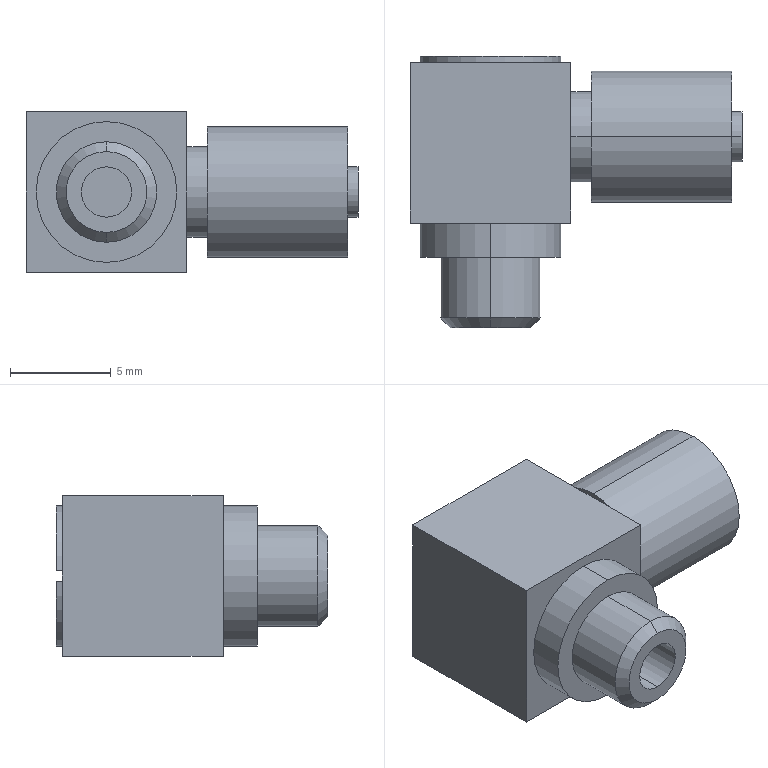Part | SolidWorks | features BaseBody 1, MoveCopyBody 1 | 1 solid | 39 faces | box 16.5 x 13.5 x 8 mm | volume 829.104 mm3 | plane 20 | cylinder 17 | cone 2 | commonest cylinder face diameters 7 x5 2.5 x4 1.8 x2 4.5 x2 5 x2 6.5 x2
STEP:
#1=CARTESIAN_POINT('',(-17.111,-6.677,-3.25));
#2=VERTEX_POINT('',#1);
#3=CARTESIAN_POINT('',(-17.111,-6.677,3.25));
#4=VERTEX_POINT('',#3);
#5=CARTESIAN_POINT('',(-17.111,-6.677,0.));
#6=DIRECTION('',(1.,0.,0.));
#7=DIRECTION('',(0.,0.,-1.));
#8=AXIS2_PLACEMENT_3D('',#5,#6,#7);
#9=CIRCLE('',#8,3.25);
#10=EDGE_CURVE('',#2,#4,#9,.T.);
#11=ORIENTED_EDGE('',*,*,#10,.T.);
#12=CARTESIAN_POINT('',(-10.111,-6.677,3.25));
#13=VERTEX_POINT('',#12);
#14=CARTESIAN_POINT('',(-13.611,-6.677,3.25));
#15=DIRECTION('',(1.,0.,0.));
#16=VECTOR('',#15,1000.);
#17=LINE('',#14,#16);
#18=EDGE_CURVE('',#4,#13,#17,.T.);
#19=ORIENTED_EDGE('',*,*,#18,.T.);
#20=CARTESIAN_POINT('',(-10.111,-6.677,-3.25));
#21=VERTEX_POINT('',#20);
#22=CARTESIAN_POINT('',(-10.111,-6.677,0.));
#23=DIRECTION('',(-1.,0.,0.));
#24=DIRECTION('',(0.,0.,-1.));
#25=AXIS2_PLACEMENT_3D('',#22,#23,#24);
#26=CIRCLE('',#25,3.25);
#27=EDGE_CURVE('',#13,#21,#26,.T.);
#28=ORIENTED_EDGE('',*,*,#27,.T.);
#29=CARTESIAN_POINT('',(-13.611,-6.677,-3.25));
#30=DIRECTION('',(1.,0.,0.));
#31=VECTOR('',#30,1000.);
#32=LINE('',#29,#31);
#33=EDGE_CURVE('',#2,#21,#32,.T.);
#34=ORIENTED_EDGE('',*,*,#33,.F.);
#35=EDGE_LOOP('',(#11,#19,#28,#34));
#36=FACE_OUTER_BOUND('',#35,.T.);
#37=CARTESIAN_POINT('',(-13.611,-6.677,0.));
#38=DIRECTION('',(1.,0.,0.));
#39=DIRECTION('',(0.,0.,-1.));
#40=AXIS2_PLACEMENT_3D('',#37,#38,#39);
#41=CYLINDRICAL_SURFACE('',#40,3.25);
#42=ADVANCED_FACE('',(#36),#41,.T.);
#43=CARTESIAN_POINT('',(-18.111,-6.677,-2.25));
#44=VERTEX_POINT('',#43);
#45=CARTESIAN_POINT('',(-18.111,-6.677,2.25));
#46=VERTEX_POINT('',#45);
#47=CARTESIAN_POINT('',(-18.111,-6.677,0.));
#48=DIRECTION('',(1.,0.,0.));
#49=DIRECTION('',(0.,0.,-1.));
#50=AXIS2_PLACEMENT_3D('',#47,#48,#49);
#51=CIRCLE('',#50,2.25);
#52=EDGE_CURVE('',#44,#46,#51,.T.);
#53=ORIENTED_EDGE('',*,*,#52,.T.);
#54=CARTESIAN_POINT('',(-17.111,-6.677,2.25));
#55=VERTEX_POINT('',#54);
#56=CARTESIAN_POINT('',(-17.611,-6.677,2.25));
#57=DIRECTION('',(1.,0.,0.));
#58=VECTOR('',#57,1000.);
#59=LINE('',#56,#58);
#60=EDGE_CURVE('',#46,#55,#59,.T.);
#61=ORIENTED_EDGE('',*,*,#60,.T.);
#62=CARTESIAN_POINT('',(-17.111,-6.677,-2.25));
#63=VERTEX_POINT('',#62);
#64=CARTESIAN_POINT('',(-17.111,-6.677,0.));
#65=DIRECTION('',(1.,0.,0.));
#66=DIRECTION('',(0.,0.,-1.));
#67=AXIS2_PLACEMENT_3D('',#64,#65,#66);
#68=CIRCLE('',#67,2.25);
#69=EDGE_CURVE('',#63,#55,#68,.T.);
#70=ORIENTED_EDGE('',*,*,#69,.F.);
#71=CARTESIAN_POINT('',(-17.611,-6.677,-2.25));
#72=DIRECTION('',(1.,0.,0.));
#73=VECTOR('',#72,1000.);
#74=LINE('',#71,#73);
#75=EDGE_CURVE('',#44,#63,#74,.T.);
#76=ORIENTED_EDGE('',*,*,#75,.F.);
#77=EDGE_LOOP('',(#53,#61,#70,#76));
#78=FACE_OUTER_BOUND('',#77,.T.);
#79=CARTESIAN_POINT('',(-17.611,-6.677,0.));
#80=DIRECTION('',(1.,0.,0.));
#81=DIRECTION('',(0.,0.,-1.));
#82=AXIS2_PLACEMENT_3D('',#79,#80,#81);
#83=CYLINDRICAL_SURFACE('',#82,2.25);
#84=ADVANCED_FACE('',(#78),#83,.T.);
#85=CARTESIAN_POINT('',(-10.111,-6.677,1.25));
#86=VERTEX_POINT('',#85);
#87=CARTESIAN_POINT('',(-10.111,-6.677,-1.25));
#88=VERTEX_POINT('',#87);
#89=CARTESIAN_POINT('',(-10.111,-6.677,0.));
#90=DIRECTION('',(-1.,0.,0.));
#91=DIRECTION('',(0.,0.,-1.));
#92=AXIS2_PLACEMENT_3D('',#89,#90,#91);
#93=CIRCLE('',#92,1.25);
#94=EDGE_CURVE('',#86,#88,#93,.T.);
#95=ORIENTED_EDGE('',*,*,#94,.F.);
#96=CARTESIAN_POINT('',(-9.611,-6.677,1.25));
#97=VERTEX_POINT('',#96);
#98=CARTESIAN_POINT('',(-9.861,-6.677,1.25));
#99=DIRECTION('',(1.,0.,0.));
#100=VECTOR('',#99,1000.);
#101=LINE('',#98,#100);
#102=EDGE_CURVE('',#86,#97,#101,.T.);
#103=ORIENTED_EDGE('',*,*,#102,.T.);
#104=CARTESIAN_POINT('',(-9.611,-6.677,-1.25));
#105=VERTEX_POINT('',#104);
#106=CARTESIAN_POINT('',(-9.611,-6.677,0.));
#107=DIRECTION('',(-1.,0.,0.));
#108=DIRECTION('',(0.,0.,-1.));
#109=AXIS2_PLACEMENT_3D('',#106,#107,#108);
#110=CIRCLE('',#109,1.25);
#111=EDGE_CURVE('',#97,#105,#110,.T.);
#112=ORIENTED_EDGE('',*,*,#111,.T.);
#113=CARTESIAN_POINT('',(-9.861,-6.677,-1.25));
#114=DIRECTION('',(1.,0.,0.));
#115=VECTOR('',#114,1000.);
#116=LINE('',#113,#115);
#117=EDGE_CURVE('',#88,#105,#116,.T.);
#118=ORIENTED_EDGE('',*,*,#117,.F.);
#119=EDGE_LOOP('',(#95,#103,#112,#118));
#120=FACE_OUTER_BOUND('',#119,.T.);
#121=CARTESIAN_POINT('',(-9.861,-6.677,0.));
#122=DIRECTION('',(1.,0.,0.));
#123=DIRECTION('',(0.,0.,-1.));
#124=AXIS2_PLACEMENT_3D('',#121,#122,#123);
#125=CYLINDRICAL_SURFACE('',#124,1.25);
#126=ADVANCED_FACE('',(#120),#125,.T.);
#127=CARTESIAN_POINT('',(-19.111,-6.677,0.9));
#128=VERTEX_POINT('',#127);
#129=CARTESIAN_POINT('',(-19.111,-6.677,-0.9));
#130=VERTEX_POINT('',#129);
#131=CARTESIAN_POINT('',(-19.111,-6.677,0.));
#132=DIRECTION('',(1.,0.,0.));
#133=DIRECTION('',(0.,0.,-1.));
#134=AXIS2_PLACEMENT_3D('',#131,#132,#133);
#135=CIRCLE('',#134,0.9);
#136=EDGE_CURVE('',#128,#130,#135,.T.);
#137=ORIENTED_EDGE('',*,*,#136,.F.);
#138=CARTESIAN_POINT('',(-9.611,-6.677,0.9));
#139=VERTEX_POINT('',#138);
#140=CARTESIAN_POINT('',(-9.611,-6.677,0.9));
#141=DIRECTION('',(1.,0.,0.));
#142=VECTOR('',#141,1000.);
#143=LINE('',#140,#142);
#144=EDGE_CURVE('',#128,#139,#143,.T.);
#145=ORIENTED_EDGE('',*,*,#144,.T.);
#146=CARTESIAN_POINT('',(-9.611,-6.677,-0.9));
#147=VERTEX_POINT('',#146);
#148=CARTESIAN_POINT('',(-9.611,-6.677,0.));
#149=DIRECTION('',(-1.,0.,0.));
#150=DIRECTION('',(0.,0.,-1.));
#151=AXIS2_PLACEMENT_3D('',#148,#149,#150);
#152=CIRCLE('',#151,0.9);
#153=EDGE_CURVE('',#147,#139,#152,.T.);
#154=ORIENTED_EDGE('',*,*,#153,.F.);
#155=CARTESIAN_POINT('',(-9.611,-6.677,-0.9));
#156=DIRECTION('',(1.,0.,0.));
#157=VECTOR('',#156,1000.);
#158=LINE('',#155,#157);
#159=EDGE_CURVE('',#130,#147,#158,.T.);
#160=ORIENTED_EDGE('',*,*,#159,.F.);
#161=EDGE_LOOP('',(#137,#145,#154,#160));
#162=FACE_OUTER_BOUND('',#161,.T.);
#163=CARTESIAN_POINT('',(-9.611,-6.677,0.));
#164=DIRECTION('',(1.,0.,0.));
#165=DIRECTION('',(0.,0.,-1.));
#166=AXIS2_PLACEMENT_3D('',#163,#164,#165);
#167=CYLINDRICAL_SURFACE('',#166,0.9);
#168=ADVANCED_FACE('',(#162),#167,.F.);
#169=CARTESIAN_POINT('',(-22.111,-10.977,-3.5));
#170=VERTEX_POINT('',#169);
#171=CARTESIAN_POINT('',(-22.111,-10.977,3.5));
#172=VERTEX_POINT('',#171);
#173=CARTESIAN_POINT('',(-22.111,-10.977,0.));
#174=DIRECTION('',(0.,-1.,0.));
#175=DIRECTION('',(0.,0.,-1.));
#176=AXIS2_PLACEMENT_3D('',#173,#174,#175);
#177=CIRCLE('',#176,3.5);
#178=EDGE_CURVE('',#170,#172,#177,.T.);
#179=ORIENTED_EDGE('',*,*,#178,.T.);
#180=CARTESIAN_POINT('',(-22.111,-12.677,3.5));
#181=VERTEX_POINT('',#180);
#182=CARTESIAN_POINT('',(-22.111,-11.827,3.5));
#183=DIRECTION('',(0.,-1.,0.));
#184=VECTOR('',#183,1000.);
#185=LINE('',#182,#184);
#186=EDGE_CURVE('',#172,#181,#185,.T.);
#187=ORIENTED_EDGE('',*,*,#186,.T.);
#188=CARTESIAN_POINT('',(-22.111,-12.677,-3.5));
#189=VERTEX_POINT('',#188);
#190=CARTESIAN_POINT('',(-22.111,-12.677,0.));
#191=DIRECTION('',(0.,1.,0.));
#192=DIRECTION('',(0.,0.,-1.));
#193=AXIS2_PLACEMENT_3D('',#190,#191,#192);
#194=CIRCLE('',#193,3.5);
#195=EDGE_CURVE('',#181,#189,#194,.T.);
#196=ORIENTED_EDGE('',*,*,#195,.T.);
#197=CARTESIAN_POINT('',(-22.111,-11.827,-3.5));
#198=DIRECTION('',(0.,-1.,0.));
#199=VECTOR('',#198,1000.);
#200=LINE('',#197,#199);
#201=EDGE_CURVE('',#170,#189,#200,.T.);
#202=ORIENTED_EDGE('',*,*,#201,.F.);
#203=EDGE_LOOP('',(#179,#187,#196,#202));
#204=FACE_OUTER_BOUND('',#203,.T.);
#205=CARTESIAN_POINT('',(-22.111,-11.827,0.));
#206=DIRECTION('',(0.,-1.,0.));
#207=DIRECTION('',(0.,0.,-1.));
#208=AXIS2_PLACEMENT_3D('',#205,#206,#207);
#209=CYLINDRICAL_SURFACE('',#208,3.5);
#210=ADVANCED_FACE('',(#204),#209,.T.);
#211=CARTESIAN_POINT('',(-25.602,-2.677,-0.25));
#212=VERTEX_POINT('',#211);
#213=CARTESIAN_POINT('',(-22.111,-2.677,-3.5));
#214=VERTEX_POINT('',#213);
#215=CARTESIAN_POINT('',(-22.111,-2.677,0.));
#216=DIRECTION('',(0.,-1.,0.));
#217=DIRECTION('',(0.,0.,-1.));
#218=AXIS2_PLACEMENT_3D('',#215,#216,#217);
#219=CIRCLE('',#218,3.5);
#220=EDGE_CURVE('',#212,#214,#219,.T.);
#221=ORIENTED_EDGE('',*,*,#220,.T.);
#222=CARTESIAN_POINT('',(-22.111,-2.977,-3.5));
#223=VERTEX_POINT('',#222);
#224=CARTESIAN_POINT('',(-22.111,-2.977,-3.5));
#225=DIRECTION('',(0.,-1.,0.));
#226=VECTOR('',#225,1000.);
#227=LINE('',#224,#226);
#228=EDGE_CURVE('',#214,#223,#227,.T.);
#229=ORIENTED_EDGE('',*,*,#228,.T.);
#230=CARTESIAN_POINT('',(-25.602,-2.977,-0.25));
#231=VERTEX_POINT('',#230);
#232=CARTESIAN_POINT('',(-22.111,-2.977,0.));
#233=DIRECTION('',(0.,-1.,0.));
#234=DIRECTION('',(0.,0.,-1.));
#235=AXIS2_PLACEMENT_3D('',#232,#233,#234);
#236=CIRCLE('',#235,3.5);
#237=EDGE_CURVE('',#231,#223,#236,.T.);
#238=ORIENTED_EDGE('',*,*,#237,.F.);
#239=CARTESIAN_POINT('',(-25.602,-2.677,-0.25));
#240=DIRECTION('',(0.,1.,0.));
#241=VECTOR('',#240,1000.);
#242=LINE('',#239,#241);
#243=EDGE_CURVE('',#231,#212,#242,.T.);
#244=ORIENTED_EDGE('',*,*,#243,.T.);
#245=EDGE_LOOP('',(#221,#229,#238,#244));
#246=FACE_OUTER_BOUND('',#245,.T.);
#247=CARTESIAN_POINT('',(-22.111,-2.977,0.));
#248=DIRECTION('',(0.,-1.,0.));
#249=DIRECTION('',(0.,0.,-1.));
#250=AXIS2_PLACEMENT_3D('',#247,#248,#249);
#251=CYLINDRICAL_SURFACE('',#250,3.5);
#252=ADVANCED_FACE('',(#246),#251,.T.);
#253=CARTESIAN_POINT('',(-22.111,-12.677,2.5));
#254=VERTEX_POINT('',#253);
#255=CARTESIAN_POINT('',(-22.111,-12.677,-2.5));
#256=VERTEX_POINT('',#255);
#257=CARTESIAN_POINT('',(-22.111,-12.677,0.));
#258=DIRECTION('',(0.,1.,0.));
#259=DIRECTION('',(0.,0.,-1.));
#260=AXIS2_PLACEMENT_3D('',#257,#258,#259);
#261=CIRCLE('',#260,2.5);
#262=EDGE_CURVE('',#254,#256,#261,.T.);
#263=ORIENTED_EDGE('',*,*,#262,.F.);
#264=CARTESIAN_POINT('',(-22.111,-15.687,2.5));
#265=VERTEX_POINT('',#264);
#266=CARTESIAN_POINT('',(-22.111,-14.182,2.5));
#267=DIRECTION('',(0.,-1.,0.));
#268=VECTOR('',#267,1000.);
#269=LINE('',#266,#268);
#270=EDGE_CURVE('',#254,#265,#269,.T.);
#271=ORIENTED_EDGE('',*,*,#270,.T.);
#272=CARTESIAN_POINT('',(-22.111,-15.687,-2.5));
#273=VERTEX_POINT('',#272);
#274=CARTESIAN_POINT('',(-22.111,-15.687,0.));
#275=DIRECTION('',(0.,1.,0.));
#276=DIRECTION('',(0.,0.,-1.));
#277=AXIS2_PLACEMENT_3D('',#274,#275,#276);
#278=CIRCLE('',#277,2.5);
#279=EDGE_CURVE('',#265,#273,#278,.T.);
#280=ORIENTED_EDGE('',*,*,#279,.T.);
#281=CARTESIAN_POINT('',(-22.111,-14.182,-2.5));
#282=DIRECTION('',(0.,-1.,0.));
#283=VECTOR('',#282,1000.);
#284=LINE('',#281,#283);
#285=EDGE_CURVE('',#256,#273,#284,.T.);
#286=ORIENTED_EDGE('',*,*,#285,.F.);
#287=EDGE_LOOP('',(#263,#271,#280,#286));
#288=FACE_OUTER_BOUND('',#287,.T.);
#289=CARTESIAN_POINT('',(-22.111,-14.182,0.));
#290=DIRECTION('',(0.,-1.,0.));
#291=DIRECTION('',(0.,0.,-1.));
#292=AXIS2_PLACEMENT_3D('',#289,#290,#291);
#293=CYLINDRICAL_SURFACE('',#292,2.5);
#294=ADVANCED_FACE('',(#288),#293,.T.);
#295=CARTESIAN_POINT('',(-22.111,-16.177,2.01));
#296=VERTEX_POINT('',#295);
#297=CARTESIAN_POINT('',(-22.111,-16.177,-2.01));
#298=VERTEX_POINT('',#297);
#299=CARTESIAN_POINT('',(-22.111,-16.177,0.));
#300=DIRECTION('',(0.,1.,0.));
#301=DIRECTION('',(0.,0.,1.));
#302=AXIS2_PLACEMENT_3D('',#299,#300,#301);
#303=CIRCLE('',#302,2.01);
#304=EDGE_CURVE('',#296,#298,#303,.T.);
#305=ORIENTED_EDGE('',*,*,#304,.T.);
#306=CARTESIAN_POINT('',(-22.111,-15.687,-2.5));
#307=DIRECTION('',(0.,0.7071,-0.7071));
#308=VECTOR('',#307,1000.);
#309=LINE('',#306,#308);
#310=EDGE_CURVE('',#298,#273,#309,.T.);
#311=ORIENTED_EDGE('',*,*,#310,.T.);
#312=ORIENTED_EDGE('',*,*,#279,.F.);
#313=CARTESIAN_POINT('',(-22.111,-15.687,2.5));
#314=DIRECTION('',(0.,0.7071,0.7071));
#315=VECTOR('',#314,1000.);
#316=LINE('',#313,#315);
#317=EDGE_CURVE('',#296,#265,#316,.T.);
#318=ORIENTED_EDGE('',*,*,#317,.F.);
#319=EDGE_LOOP('',(#305,#311,#312,#318));
#320=FACE_OUTER_BOUND('',#319,.T.);
#321=CARTESIAN_POINT('',(-22.111,-15.687,0.));
#322=DIRECTION('',(0.,1.,0.));
#323=DIRECTION('',(0.,0.,1.));
#324=AXIS2_PLACEMENT_3D('',#321,#322,#323);
#325=CONICAL_SURFACE('',#324,2.5,0.7854);
#326=ADVANCED_FACE('',(#320),#325,.T.);
#327=CARTESIAN_POINT('',(-22.111,-5.677,1.25));
#328=VERTEX_POINT('',#327);
#329=CARTESIAN_POINT('',(-22.111,-5.677,-1.25));
#330=VERTEX_POINT('',#329);
#331=CARTESIAN_POINT('',(-22.111,-5.677,0.));
#332=DIRECTION('',(0.,-1.,0.));
#333=DIRECTION('',(0.,0.,-1.));
#334=AXIS2_PLACEMENT_3D('',#331,#332,#333);
#335=CIRCLE('',#334,1.25);
#336=EDGE_CURVE('',#328,#330,#335,.T.);
#337=ORIENTED_EDGE('',*,*,#336,.F.);
#338=CARTESIAN_POINT('',(-22.111,-16.177,1.25));
#339=VERTEX_POINT('',#338);
#340=CARTESIAN_POINT('',(-22.111,-16.177,1.25));
#341=DIRECTION('',(0.,-1.,0.));
#342=VECTOR('',#341,1000.);
#343=LINE('',#340,#342);
#344=EDGE_CURVE('',#328,#339,#343,.T.);
#345=ORIENTED_EDGE('',*,*,#344,.T.);
#346=CARTESIAN_POINT('',(-22.111,-16.177,-1.25));
#347=VERTEX_POINT('',#346);
#348=CARTESIAN_POINT('',(-22.111,-16.177,0.));
#349=DIRECTION('',(0.,1.,0.));
#350=DIRECTION('',(0.,0.,-1.));
#351=AXIS2_PLACEMENT_3D('',#348,#349,#350);
#352=CIRCLE('',#351,1.25);
#353=EDGE_CURVE('',#347,#339,#352,.T.);
#354=ORIENTED_EDGE('',*,*,#353,.F.);
#355=CARTESIAN_POINT('',(-22.111,-16.177,-1.25));
#356=DIRECTION('',(0.,-1.,0.));
#357=VECTOR('',#356,1000.);
#358=LINE('',#355,#357);
#359=EDGE_CURVE('',#330,#347,#358,.T.);
#360=ORIENTED_EDGE('',*,*,#359,.F.);
#361=EDGE_LOOP('',(#337,#345,#354,#360));
#362=FACE_OUTER_BOUND('',#361,.T.);
#363=CARTESIAN_POINT('',(-22.111,-16.177,0.));
#364=DIRECTION('',(0.,-1.,0.));
#365=DIRECTION('',(0.,0.,-1.));
#366=AXIS2_PLACEMENT_3D('',#363,#364,#365);
#367=CYLINDRICAL_SURFACE('',#366,1.25);
#368=ADVANCED_FACE('',(#362),#367,.F.);
#369=ORIENTED_EDGE('',*,*,#18,.F.);
#370=CARTESIAN_POINT('',(-17.111,-6.677,0.));
#371=DIRECTION('',(1.,0.,0.));
#372=DIRECTION('',(0.,0.,-1.));
#373=AXIS2_PLACEMENT_3D('',#370,#371,#372);
#374=CIRCLE('',#373,3.25);
#375=EDGE_CURVE('',#4,#2,#374,.T.);
#376=ORIENTED_EDGE('',*,*,#375,.T.);
#377=ORIENTED_EDGE('',*,*,#33,.T.);
#378=CARTESIAN_POINT('',(-10.111,-6.677,0.));
#379=DIRECTION('',(-1.,0.,0.));
#380=DIRECTION('',(0.,0.,-1.));
#381=AXIS2_PLACEMENT_3D('',#378,#379,#380);
#382=CIRCLE('',#381,3.25);
#383=EDGE_CURVE('',#21,#13,#382,.T.);
#384=ORIENTED_EDGE('',*,*,#383,.T.);
#385=EDGE_LOOP('',(#369,#376,#377,#384));
#386=FACE_OUTER_BOUND('',#385,.T.);
#387=CARTESIAN_POINT('',(-13.611,-6.677,0.));
#388=DIRECTION('',(1.,0.,0.));
#389=DIRECTION('',(0.,0.,-1.));
#390=AXIS2_PLACEMENT_3D('',#387,#388,#389);
#391=CYLINDRICAL_SURFACE('',#390,3.25);
#392=ADVANCED_FACE('',(#386),#391,.T.);
#393=ORIENTED_EDGE('',*,*,#10,.F.);
#394=ORIENTED_EDGE('',*,*,#375,.F.);
#395=EDGE_LOOP('',(#393,#394));
#396=FACE_OUTER_BOUND('',#395,.T.);
#397=ORIENTED_EDGE('',*,*,#69,.T.);
#398=CARTESIAN_POINT('',(-17.111,-6.677,0.));
#399=DIRECTION('',(1.,0.,0.));
#400=DIRECTION('',(0.,0.,-1.));
#401=AXIS2_PLACEMENT_3D('',#398,#399,#400);
#402=CIRCLE('',#401,2.25);
#403=EDGE_CURVE('',#55,#63,#402,.T.);
#404=ORIENTED_EDGE('',*,*,#403,.T.);
#405=EDGE_LOOP('',(#397,#404));
#406=FACE_BOUND('',#405,.T.);
#407=CARTESIAN_POINT('',(-17.111,-3.927,0.));
#408=DIRECTION('',(-1.,0.,0.));
#409=DIRECTION('',(0.,0.,1.));
#410=AXIS2_PLACEMENT_3D('',#407,#408,#409);
#411=PLANE('',#410);
#412=ADVANCED_FACE('',(#396,#406),#411,.T.);
#413=CARTESIAN_POINT('',(-10.111,-6.677,0.));
#414=DIRECTION('',(-1.,0.,0.));
#415=DIRECTION('',(0.,0.,-1.));
#416=AXIS2_PLACEMENT_3D('',#413,#414,#415);
#417=CIRCLE('',#416,1.25);
#418=EDGE_CURVE('',#88,#86,#417,.T.);
#419=ORIENTED_EDGE('',*,*,#418,.T.);
#420=ORIENTED_EDGE('',*,*,#94,.T.);
#421=EDGE_LOOP('',(#419,#420));
#422=FACE_BOUND('',#421,.T.);
#423=ORIENTED_EDGE('',*,*,#383,.F.);
#424=ORIENTED_EDGE('',*,*,#27,.F.);
#425=EDGE_LOOP('',(#423,#424));
#426=FACE_OUTER_BOUND('',#425,.T.);
#427=CARTESIAN_POINT('',(-10.111,-4.427,0.));
#428=DIRECTION('',(1.,0.,0.));
#429=DIRECTION('',(0.,0.,-1.));
#430=AXIS2_PLACEMENT_3D('',#427,#428,#429);
#431=PLANE('',#430);
#432=ADVANCED_FACE('',(#422,#426),#431,.T.);
#433=ORIENTED_EDGE('',*,*,#60,.F.);
#434=CARTESIAN_POINT('',(-18.111,-6.677,0.));
#435=DIRECTION('',(1.,0.,0.));
#436=DIRECTION('',(0.,0.,-1.));
#437=AXIS2_PLACEMENT_3D('',#434,#435,#436);
#438=CIRCLE('',#437,2.25);
#439=EDGE_CURVE('',#46,#44,#438,.T.);
#440=ORIENTED_EDGE('',*,*,#439,.T.);
#441=ORIENTED_EDGE('',*,*,#75,.T.);
#442=ORIENTED_EDGE('',*,*,#403,.F.);
#443=EDGE_LOOP('',(#433,#440,#441,#442));
#444=FACE_OUTER_BOUND('',#443,.T.);
#445=CARTESIAN_POINT('',(-17.611,-6.677,0.));
#446=DIRECTION('',(1.,0.,0.));
#447=DIRECTION('',(0.,0.,-1.));
#448=AXIS2_PLACEMENT_3D('',#445,#446,#447);
#449=CYLINDRICAL_SURFACE('',#448,2.25);
#450=ADVANCED_FACE('',(#444),#449,.T.);
#451=ORIENTED_EDGE('',*,*,#102,.F.);
#452=ORIENTED_EDGE('',*,*,#418,.F.);
#453=ORIENTED_EDGE('',*,*,#117,.T.);
#454=CARTESIAN_POINT('',(-9.611,-6.677,0.));
#455=DIRECTION('',(-1.,0.,0.));
#456=DIRECTION('',(0.,0.,-1.));
#457=AXIS2_PLACEMENT_3D('',#454,#455,#456);
#458=CIRCLE('',#457,1.25);
#459=EDGE_CURVE('',#105,#97,#458,.T.);
#460=ORIENTED_EDGE('',*,*,#459,.T.);
#461=EDGE_LOOP('',(#451,#452,#453,#460));
#462=FACE_OUTER_BOUND('',#461,.T.);
#463=CARTESIAN_POINT('',(-9.861,-6.677,0.));
#464=DIRECTION('',(1.,0.,0.));
#465=DIRECTION('',(0.,0.,-1.));
#466=AXIS2_PLACEMENT_3D('',#463,#464,#465);
#467=CYLINDRICAL_SURFACE('',#466,1.25);
#468=ADVANCED_FACE('',(#462),#467,.T.);
#469=CARTESIAN_POINT('',(-18.111,-10.977,4.));
#470=VERTEX_POINT('',#469);
#471=CARTESIAN_POINT('',(-18.111,-10.977,-4.));
#472=VERTEX_POINT('',#471);
#473=CARTESIAN_POINT('',(-18.111,-10.977,-4.));
#474=DIRECTION('',(0.,0.,-1.));
#475=VECTOR('',#474,1000.);
#476=LINE('',#473,#475);
#477=EDGE_CURVE('',#470,#472,#476,.T.);
#478=ORIENTED_EDGE('',*,*,#477,.T.);
#479=CARTESIAN_POINT('',(-18.111,-2.977,-4.));
#480=VERTEX_POINT('',#479);
#481=CARTESIAN_POINT('',(-18.111,-10.977,-4.));
#482=DIRECTION('',(0.,1.,0.));
#483=VECTOR('',#482,1000.);
#484=LINE('',#481,#483);
#485=EDGE_CURVE('',#472,#480,#484,.T.);
#486=ORIENTED_EDGE('',*,*,#485,.T.);
#487=CARTESIAN_POINT('',(-18.111,-2.977,4.));
#488=VERTEX_POINT('',#487);
#489=CARTESIAN_POINT('',(-18.111,-2.977,-4.));
#490=DIRECTION('',(0.,0.,1.));
#491=VECTOR('',#490,1000.);
#492=LINE('',#489,#491);
#493=EDGE_CURVE('',#480,#488,#492,.T.);
#494=ORIENTED_EDGE('',*,*,#493,.T.);
#495=CARTESIAN_POINT('',(-18.111,-10.977,4.));
#496=DIRECTION('',(0.,-1.,0.));
#497=VECTOR('',#496,1000.);
#498=LINE('',#495,#497);
#499=EDGE_CURVE('',#488,#470,#498,.T.);
#500=ORIENTED_EDGE('',*,*,#499,.T.);
#501=EDGE_LOOP('',(#478,#486,#494,#500));
#502=FACE_OUTER_BOUND('',#501,.T.);
#503=ORIENTED_EDGE('',*,*,#52,.F.);
#504=ORIENTED_EDGE('',*,*,#439,.F.);
#505=EDGE_LOOP('',(#503,#504));
#506=FACE_BOUND('',#505,.T.);
#507=CARTESIAN_POINT('',(-18.111,-10.977,-4.));
#508=DIRECTION('',(1.,0.,0.));
#509=DIRECTION('',(0.,0.,-1.));
#510=AXIS2_PLACEMENT_3D('',#507,#508,#509);
#511=PLANE('',#510);
#512=ADVANCED_FACE('',(#502,#506),#511,.T.);
#513=ORIENTED_EDGE('',*,*,#459,.F.);
#514=ORIENTED_EDGE('',*,*,#111,.F.);
#515=EDGE_LOOP('',(#513,#514));
#516=FACE_OUTER_BOUND('',#515,.T.);
#517=ORIENTED_EDGE('',*,*,#153,.T.);
#518=CARTESIAN_POINT('',(-9.611,-6.677,0.));
#519=DIRECTION('',(-1.,0.,0.));
#520=DIRECTION('',(0.,0.,-1.));
#521=AXIS2_PLACEMENT_3D('',#518,#519,#520);
#522=CIRCLE('',#521,0.9);
#523=EDGE_CURVE('',#139,#147,#522,.T.);
#524=ORIENTED_EDGE('',*,*,#523,.T.);
#525=EDGE_LOOP('',(#517,#524));
#526=FACE_BOUND('',#525,.T.);
#527=CARTESIAN_POINT('',(-9.611,-6.052,0.));
#528=DIRECTION('',(1.,0.,0.));
#529=DIRECTION('',(0.,0.,-1.));
#530=AXIS2_PLACEMENT_3D('',#527,#528,#529);
#531=PLANE('',#530);
#532=ADVANCED_FACE('',(#516,#526),#531,.T.);
#533=CARTESIAN_POINT('',(-26.111,-10.977,-4.));
#534=VERTEX_POINT('',#533);
#535=CARTESIAN_POINT('',(-26.111,-10.977,-4.));
#536=DIRECTION('',(-1.,0.,0.));
#537=VECTOR('',#536,1000.);
#538=LINE('',#535,#537);
#539=EDGE_CURVE('',#472,#534,#538,.T.);
#540=ORIENTED_EDGE('',*,*,#539,.T.);
#541=CARTESIAN_POINT('',(-26.111,-2.977,-4.));
#542=VERTEX_POINT('',#541);
#543=CARTESIAN_POINT('',(-26.111,-10.977,-4.));
#544=DIRECTION('',(0.,1.,0.));
#545=VECTOR('',#544,1000.);
#546=LINE('',#543,#545);
#547=EDGE_CURVE('',#534,#542,#546,.T.);
#548=ORIENTED_EDGE('',*,*,#547,.T.);
#549=CARTESIAN_POINT('',(-26.111,-2.977,-4.));
#550=DIRECTION('',(1.,0.,0.));
#551=VECTOR('',#550,1000.);
#552=LINE('',#549,#551);
#553=EDGE_CURVE('',#542,#480,#552,.T.);
#554=ORIENTED_EDGE('',*,*,#553,.T.);
#555=ORIENTED_EDGE('',*,*,#485,.F.);
#556=EDGE_LOOP('',(#540,#548,#554,#555));
#557=FACE_OUTER_BOUND('',#556,.T.);
#558=CARTESIAN_POINT('',(-26.111,-10.977,-4.));
#559=DIRECTION('',(0.,0.,-1.));
#560=DIRECTION('',(-1.,0.,0.));
#561=AXIS2_PLACEMENT_3D('',#558,#559,#560);
#562=PLANE('',#561);
#563=ADVANCED_FACE('',(#557),#562,.T.);
#564=ORIENTED_EDGE('',*,*,#178,.F.);
#565=CARTESIAN_POINT('',(-22.111,-10.977,0.));
#566=DIRECTION('',(0.,-1.,0.));
#567=DIRECTION('',(0.,0.,-1.));
#568=AXIS2_PLACEMENT_3D('',#565,#566,#567);
#569=CIRCLE('',#568,3.5);
#570=EDGE_CURVE('',#172,#170,#569,.T.);
#571=ORIENTED_EDGE('',*,*,#570,.F.);
#572=EDGE_LOOP('',(#564,#571));
#573=FACE_BOUND('',#572,.T.);
#574=ORIENTED_EDGE('',*,*,#539,.F.);
#575=ORIENTED_EDGE('',*,*,#477,.F.);
#576=CARTESIAN_POINT('',(-26.111,-10.977,4.));
#577=VERTEX_POINT('',#576);
#578=CARTESIAN_POINT('',(-22.111,-10.977,4.));
#579=DIRECTION('',(1.,0.,0.));
#580=VECTOR('',#579,1000.);
#581=LINE('',#578,#580);
#582=EDGE_CURVE('',#577,#470,#581,.T.);
#583=ORIENTED_EDGE('',*,*,#582,.F.);
#584=CARTESIAN_POINT('',(-26.111,-10.977,0.));
#585=DIRECTION('',(0.,0.,1.));
#586=VECTOR('',#585,1000.);
#587=LINE('',#584,#586);
#588=EDGE_CURVE('',#534,#577,#587,.T.);
#589=ORIENTED_EDGE('',*,*,#588,.F.);
#590=EDGE_LOOP('',(#574,#575,#583,#589));
#591=FACE_OUTER_BOUND('',#590,.T.);
#592=CARTESIAN_POINT('',(-22.111,-10.977,0.));
#593=DIRECTION('',(0.,1.,0.));
#594=DIRECTION('',(0.,0.,1.));
#595=AXIS2_PLACEMENT_3D('',#592,#593,#594);
#596=PLANE('',#595);
#597=ADVANCED_FACE('',(#573,#591),#596,.F.);
#598=ORIENTED_EDGE('',*,*,#582,.T.);
#599=ORIENTED_EDGE('',*,*,#499,.F.);
#600=CARTESIAN_POINT('',(-26.111,-2.977,4.));
#601=VERTEX_POINT('',#600);
#602=CARTESIAN_POINT('',(-18.111,-2.977,4.));
#603=DIRECTION('',(-1.,0.,0.));
#604=VECTOR('',#603,1000.);
#605=LINE('',#602,#604);
#606=EDGE_CURVE('',#488,#601,#605,.T.);
#607=ORIENTED_EDGE('',*,*,#606,.T.);
#608=CARTESIAN_POINT('',(-26.111,-10.977,4.));
#609=DIRECTION('',(0.,-1.,0.));
#610=VECTOR('',#609,1000.);
#611=LINE('',#608,#610);
#612=EDGE_CURVE('',#601,#577,#611,.T.);
#613=ORIENTED_EDGE('',*,*,#612,.T.);
#614=EDGE_LOOP('',(#598,#599,#607,#613));
#615=FACE_OUTER_BOUND('',#614,.T.);
#616=CARTESIAN_POINT('',(-18.111,-10.977,4.));
#617=DIRECTION('',(0.,0.,1.));
#618=DIRECTION('',(1.,0.,0.));
#619=AXIS2_PLACEMENT_3D('',#616,#617,#618);
#620=PLANE('',#619);
#621=ADVANCED_FACE('',(#615),#620,.T.);
#622=ORIENTED_EDGE('',*,*,#606,.F.);
#623=ORIENTED_EDGE('',*,*,#493,.F.);
#624=ORIENTED_EDGE('',*,*,#553,.F.);
#625=CARTESIAN_POINT('',(-26.111,-2.977,0.));
#626=DIRECTION('',(0.,0.,1.));
#627=VECTOR('',#626,1000.);
#628=LINE('',#625,#627);
#629=EDGE_CURVE('',#542,#601,#628,.T.);
#630=ORIENTED_EDGE('',*,*,#629,.T.);
#631=EDGE_LOOP('',(#622,#623,#624,#630));
#632=FACE_OUTER_BOUND('',#631,.T.);
#633=CARTESIAN_POINT('',(-25.611,-2.977,-0.25));
#634=VERTEX_POINT('',#633);
#635=CARTESIAN_POINT('',(-18.611,-2.977,-0.25));
#636=DIRECTION('',(1.,0.,0.));
#637=VECTOR('',#636,1000.);
#638=LINE('',#635,#637);
#639=EDGE_CURVE('',#634,#231,#638,.T.);
#640=ORIENTED_EDGE('',*,*,#639,.T.);
#641=ORIENTED_EDGE('',*,*,#237,.T.);
#642=CARTESIAN_POINT('',(-18.62,-2.977,-0.25));
#643=VERTEX_POINT('',#642);
#644=CARTESIAN_POINT('',(-22.111,-2.977,0.));
#645=DIRECTION('',(0.,-1.,0.));
#646=DIRECTION('',(0.,0.,-1.));
#647=AXIS2_PLACEMENT_3D('',#644,#645,#646);
#648=CIRCLE('',#647,3.5);
#649=EDGE_CURVE('',#223,#643,#648,.T.);
#650=ORIENTED_EDGE('',*,*,#649,.T.);
#651=CARTESIAN_POINT('',(-18.611,-2.977,-0.25));
#652=VERTEX_POINT('',#651);
#653=CARTESIAN_POINT('',(-18.611,-2.977,-0.25));
#654=DIRECTION('',(1.,0.,0.));
#655=VECTOR('',#654,1000.);
#656=LINE('',#653,#655);
#657=EDGE_CURVE('',#643,#652,#656,.T.);
#658=ORIENTED_EDGE('',*,*,#657,.T.);
#659=CARTESIAN_POINT('',(-18.611,-2.977,0.25));
#660=VERTEX_POINT('',#659);
#661=CARTESIAN_POINT('',(-18.611,-2.977,0.));
#662=DIRECTION('',(0.,0.,1.));
#663=VECTOR('',#662,1000.);
#664=LINE('',#661,#663);
#665=EDGE_CURVE('',#652,#660,#664,.T.);
#666=ORIENTED_EDGE('',*,*,#665,.T.);
#667=CARTESIAN_POINT('',(-18.62,-2.977,0.25));
#668=VERTEX_POINT('',#667);
#669=CARTESIAN_POINT('',(-25.611,-2.977,0.25));
#670=DIRECTION('',(-1.,0.,0.));
#671=VECTOR('',#670,1000.);
#672=LINE('',#669,#671);
#673=EDGE_CURVE('',#660,#668,#672,.T.);
#674=ORIENTED_EDGE('',*,*,#673,.T.);
#675=CARTESIAN_POINT('',(-25.602,-2.977,0.25));
#676=VERTEX_POINT('',#675);
#677=CARTESIAN_POINT('',(-22.111,-2.977,0.));
#678=DIRECTION('',(0.,-1.,0.));
#679=DIRECTION('',(0.,0.,-1.));
#680=AXIS2_PLACEMENT_3D('',#677,#678,#679);
#681=CIRCLE('',#680,3.5);
#682=EDGE_CURVE('',#668,#676,#681,.T.);
#683=ORIENTED_EDGE('',*,*,#682,.T.);
#684=CARTESIAN_POINT('',(-25.611,-2.977,0.25));
#685=VERTEX_POINT('',#684);
#686=CARTESIAN_POINT('',(-25.611,-2.977,0.25));
#687=DIRECTION('',(-1.,0.,0.));
#688=VECTOR('',#687,1000.);
#689=LINE('',#686,#688);
#690=EDGE_CURVE('',#676,#685,#689,.T.);
#691=ORIENTED_EDGE('',*,*,#690,.T.);
#692=CARTESIAN_POINT('',(-25.611,-2.977,0.));
#693=DIRECTION('',(0.,0.,-1.));
#694=VECTOR('',#693,1000.);
#695=LINE('',#692,#694);
#696=EDGE_CURVE('',#685,#634,#695,.T.);
#697=ORIENTED_EDGE('',*,*,#696,.T.);
#698=EDGE_LOOP('',(#640,#641,#650,#658,#666,#674,#683,#691,#697));
#699=FACE_BOUND('',#698,.T.);
#700=CARTESIAN_POINT('',(-22.111,-2.977,0.));
#701=DIRECTION('',(0.,1.,0.));
#702=DIRECTION('',(0.,0.,1.));
#703=AXIS2_PLACEMENT_3D('',#700,#701,#702);
#704=PLANE('',#703);
#705=ADVANCED_FACE('',(#632,#699),#704,.T.);
#706=ORIENTED_EDGE('',*,*,#144,.F.);
#707=CARTESIAN_POINT('',(-19.111,-6.677,0.));
#708=DIRECTION('',(1.,0.,0.));
#709=DIRECTION('',(0.,0.,-1.));
#710=AXIS2_PLACEMENT_3D('',#707,#708,#709);
#711=CIRCLE('',#710,0.9);
#712=EDGE_CURVE('',#130,#128,#711,.T.);
#713=ORIENTED_EDGE('',*,*,#712,.F.);
#714=ORIENTED_EDGE('',*,*,#159,.T.);
#715=ORIENTED_EDGE('',*,*,#523,.F.);
#716=EDGE_LOOP('',(#706,#713,#714,#715));
#717=FACE_OUTER_BOUND('',#716,.T.);
#718=CARTESIAN_POINT('',(-9.611,-6.677,0.));
#719=DIRECTION('',(1.,0.,0.));
#720=DIRECTION('',(0.,0.,-1.));
#721=AXIS2_PLACEMENT_3D('',#718,#719,#720);
#722=CYLINDRICAL_SURFACE('',#721,0.9);
#723=ADVANCED_FACE('',(#717),#722,.F.);
#724=ORIENTED_EDGE('',*,*,#588,.T.);
#725=ORIENTED_EDGE('',*,*,#612,.F.);
#726=ORIENTED_EDGE('',*,*,#629,.F.);
#727=ORIENTED_EDGE('',*,*,#547,.F.);
#728=EDGE_LOOP('',(#724,#725,#726,#727));
#729=FACE_OUTER_BOUND('',#728,.T.);
#730=CARTESIAN_POINT('',(-26.111,-10.977,4.));
#731=DIRECTION('',(-1.,0.,0.));
#732=DIRECTION('',(0.,0.,1.));
#733=AXIS2_PLACEMENT_3D('',#730,#731,#732);
#734=PLANE('',#733);
#735=ADVANCED_FACE('',(#729),#734,.T.);
#736=ORIENTED_EDGE('',*,*,#186,.F.);
#737=ORIENTED_EDGE('',*,*,#570,.T.);
#738=ORIENTED_EDGE('',*,*,#201,.T.);
#739=CARTESIAN_POINT('',(-22.111,-12.677,0.));
#740=DIRECTION('',(0.,1.,0.));
#741=DIRECTION('',(0.,0.,-1.));
#742=AXIS2_PLACEMENT_3D('',#739,#740,#741);
#743=CIRCLE('',#742,3.5);
#744=EDGE_CURVE('',#189,#181,#743,.T.);
#745=ORIENTED_EDGE('',*,*,#744,.T.);
#746=EDGE_LOOP('',(#736,#737,#738,#745));
#747=FACE_OUTER_BOUND('',#746,.T.);
#748=CARTESIAN_POINT('',(-22.111,-11.827,0.));
#749=DIRECTION('',(0.,-1.,0.));
#750=DIRECTION('',(0.,0.,-1.));
#751=AXIS2_PLACEMENT_3D('',#748,#749,#750);
#752=CYLINDRICAL_SURFACE('',#751,3.5);
#753=ADVANCED_FACE('',(#747),#752,.T.);
#754=ORIENTED_EDGE('',*,*,#228,.F.);
#755=CARTESIAN_POINT('',(-18.62,-2.677,-0.25));
#756=VERTEX_POINT('',#755);
#757=CARTESIAN_POINT('',(-22.111,-2.677,0.));
#758=DIRECTION('',(0.,-1.,0.));
#759=DIRECTION('',(0.,0.,-1.));
#760=AXIS2_PLACEMENT_3D('',#757,#758,#759);
#761=CIRCLE('',#760,3.5);
#762=EDGE_CURVE('',#214,#756,#761,.T.);
#763=ORIENTED_EDGE('',*,*,#762,.T.);
#764=CARTESIAN_POINT('',(-18.62,-2.677,-0.25));
#765=DIRECTION('',(0.,-1.,0.));
#766=VECTOR('',#765,1000.);
#767=LINE('',#764,#766);
#768=EDGE_CURVE('',#756,#643,#767,.T.);
#769=ORIENTED_EDGE('',*,*,#768,.T.);
#770=ORIENTED_EDGE('',*,*,#649,.F.);
#771=EDGE_LOOP('',(#754,#763,#769,#770));
#772=FACE_OUTER_BOUND('',#771,.T.);
#773=CARTESIAN_POINT('',(-22.111,-2.977,0.));
#774=DIRECTION('',(0.,-1.,0.));
#775=DIRECTION('',(0.,0.,-1.));
#776=AXIS2_PLACEMENT_3D('',#773,#774,#775);
#777=CYLINDRICAL_SURFACE('',#776,3.5);
#778=ADVANCED_FACE('',(#772),#777,.T.);
#779=CARTESIAN_POINT('',(-25.611,-3.177,0.25));
#780=VERTEX_POINT('',#779);
#781=CARTESIAN_POINT('',(-25.611,-2.677,0.25));
#782=DIRECTION('',(0.,-1.,0.));
#783=VECTOR('',#782,1000.);
#784=LINE('',#781,#783);
#785=EDGE_CURVE('',#685,#780,#784,.T.);
#786=ORIENTED_EDGE('',*,*,#785,.T.);
#787=CARTESIAN_POINT('',(-25.611,-3.177,-0.25));
#788=VERTEX_POINT('',#787);
#789=CARTESIAN_POINT('',(-25.611,-3.177,0.));
#790=DIRECTION('',(0.,0.,1.));
#791=VECTOR('',#790,1000.);
#792=LINE('',#789,#791);
#793=EDGE_CURVE('',#788,#780,#792,.T.);
#794=ORIENTED_EDGE('',*,*,#793,.F.);
#795=CARTESIAN_POINT('',(-25.611,-2.677,-0.25));
#796=DIRECTION('',(0.,1.,0.));
#797=VECTOR('',#796,1000.);
#798=LINE('',#795,#797);
#799=EDGE_CURVE('',#788,#634,#798,.T.);
#800=ORIENTED_EDGE('',*,*,#799,.T.);
#801=ORIENTED_EDGE('',*,*,#696,.F.);
#802=EDGE_LOOP('',(#786,#794,#800,#801));
#803=FACE_OUTER_BOUND('',#802,.T.);
#804=CARTESIAN_POINT('',(-25.611,-2.677,-0.25));
#805=DIRECTION('',(-1.,0.,0.));
#806=DIRECTION('',(0.,0.,1.));
#807=AXIS2_PLACEMENT_3D('',#804,#805,#806);
#808=PLANE('',#807);
#809=ADVANCED_FACE('',(#803),#808,.F.);
#810=CARTESIAN_POINT('',(-25.602,-2.677,0.25));
#811=VERTEX_POINT('',#810);
#812=CARTESIAN_POINT('',(-25.602,-2.677,0.25));
#813=DIRECTION('',(0.,-1.,0.));
#814=VECTOR('',#813,1000.);
#815=LINE('',#812,#814);
#816=EDGE_CURVE('',#811,#676,#815,.T.);
#817=ORIENTED_EDGE('',*,*,#816,.T.);
#818=ORIENTED_EDGE('',*,*,#682,.F.);
#819=CARTESIAN_POINT('',(-18.62,-2.677,0.25));
#820=VERTEX_POINT('',#819);
#821=CARTESIAN_POINT('',(-18.62,-2.677,0.25));
#822=DIRECTION('',(0.,1.,0.));
#823=VECTOR('',#822,1000.);
#824=LINE('',#821,#823);
#825=EDGE_CURVE('',#668,#820,#824,.T.);
#826=ORIENTED_EDGE('',*,*,#825,.T.);
#827=CARTESIAN_POINT('',(-22.111,-2.677,0.));
#828=DIRECTION('',(0.,-1.,0.));
#829=DIRECTION('',(0.,0.,-1.));
#830=AXIS2_PLACEMENT_3D('',#827,#828,#829);
#831=CIRCLE('',#830,3.5);
#832=EDGE_CURVE('',#820,#811,#831,.T.);
#833=ORIENTED_EDGE('',*,*,#832,.T.);
#834=EDGE_LOOP('',(#817,#818,#826,#833));
#835=FACE_OUTER_BOUND('',#834,.T.);
#836=CARTESIAN_POINT('',(-22.111,-2.977,0.));
#837=DIRECTION('',(0.,-1.,0.));
#838=DIRECTION('',(0.,0.,-1.));
#839=AXIS2_PLACEMENT_3D('',#836,#837,#838);
#840=CYLINDRICAL_SURFACE('',#839,3.5);
#841=ADVANCED_FACE('',(#835),#840,.T.);
#842=CARTESIAN_POINT('',(-18.611,-3.177,-0.25));
#843=VERTEX_POINT('',#842);
#844=CARTESIAN_POINT('',(-18.611,-2.677,-0.25));
#845=DIRECTION('',(0.,-1.,0.));
#846=VECTOR('',#845,1000.);
#847=LINE('',#844,#846);
#848=EDGE_CURVE('',#652,#843,#847,.T.);
#849=ORIENTED_EDGE('',*,*,#848,.T.);
#850=CARTESIAN_POINT('',(-18.611,-3.177,0.25));
#851=VERTEX_POINT('',#850);
#852=CARTESIAN_POINT('',(-18.611,-3.177,0.));
#853=DIRECTION('',(0.,0.,-1.));
#854=VECTOR('',#853,1000.);
#855=LINE('',#852,#854);
#856=EDGE_CURVE('',#851,#843,#855,.T.);
#857=ORIENTED_EDGE('',*,*,#856,.F.);
#858=CARTESIAN_POINT('',(-18.611,-2.677,0.25));
#859=DIRECTION('',(0.,1.,0.));
#860=VECTOR('',#859,1000.);
#861=LINE('',#858,#860);
#862=EDGE_CURVE('',#851,#660,#861,.T.);
#863=ORIENTED_EDGE('',*,*,#862,.T.);
#864=ORIENTED_EDGE('',*,*,#665,.F.);
#865=EDGE_LOOP('',(#849,#857,#863,#864));
#866=FACE_OUTER_BOUND('',#865,.T.);
#867=CARTESIAN_POINT('',(-18.611,-2.677,0.25));
#868=DIRECTION('',(1.,0.,0.));
#869=DIRECTION('',(0.,0.,-1.));
#870=AXIS2_PLACEMENT_3D('',#867,#868,#869);
#871=PLANE('',#870);
#872=ADVANCED_FACE('',(#866),#871,.F.);
#873=ORIENTED_EDGE('',*,*,#712,.T.);
#874=ORIENTED_EDGE('',*,*,#136,.T.);
#875=EDGE_LOOP('',(#873,#874));
#876=FACE_OUTER_BOUND('',#875,.T.);
#877=CARTESIAN_POINT('',(-19.111,-6.677,0.));
#878=DIRECTION('',(1.,0.,0.));
#879=DIRECTION('',(0.,0.,-1.));
#880=AXIS2_PLACEMENT_3D('',#877,#878,#879);
#881=PLANE('',#880);
#882=ADVANCED_FACE('',(#876),#881,.T.);
#883=CARTESIAN_POINT('',(-22.111,-12.677,0.));
#884=DIRECTION('',(0.,1.,0.));
#885=DIRECTION('',(0.,0.,-1.));
#886=AXIS2_PLACEMENT_3D('',#883,#884,#885);
#887=CIRCLE('',#886,2.5);
#888=EDGE_CURVE('',#256,#254,#887,.T.);
#889=ORIENTED_EDGE('',*,*,#888,.T.);
#890=ORIENTED_EDGE('',*,*,#262,.T.);
#891=EDGE_LOOP('',(#889,#890));
#892=FACE_BOUND('',#891,.T.);
#893=ORIENTED_EDGE('',*,*,#744,.F.);
#894=ORIENTED_EDGE('',*,*,#195,.F.);
#895=EDGE_LOOP('',(#893,#894));
#896=FACE_OUTER_BOUND('',#895,.T.);
#897=CARTESIAN_POINT('',(-19.111,-12.677,0.));
#898=DIRECTION('',(0.,-1.,0.));
#899=DIRECTION('',(0.,0.,-1.));
#900=AXIS2_PLACEMENT_3D('',#897,#898,#899);
#901=PLANE('',#900);
#902=ADVANCED_FACE('',(#892,#896),#901,.T.);
#903=CARTESIAN_POINT('',(-26.111,-2.677,-0.25));
#904=DIRECTION('',(1.,0.,0.));
#905=VECTOR('',#904,1000.);
#906=LINE('',#903,#905);
#907=EDGE_CURVE('',#212,#756,#906,.T.);
#908=ORIENTED_EDGE('',*,*,#907,.T.);
#909=ORIENTED_EDGE('',*,*,#762,.F.);
#910=ORIENTED_EDGE('',*,*,#220,.F.);
#911=EDGE_LOOP('',(#908,#909,#910));
#912=FACE_OUTER_BOUND('',#911,.T.);
#913=CARTESIAN_POINT('',(-26.111,-2.677,4.));
#914=DIRECTION('',(0.,1.,0.));
#915=DIRECTION('',(0.,0.,1.));
#916=AXIS2_PLACEMENT_3D('',#913,#914,#915);
#917=PLANE('',#916);
#918=ADVANCED_FACE('',(#912),#917,.T.);
#919=CARTESIAN_POINT('',(-26.111,-2.677,0.25));
#920=DIRECTION('',(-1.,0.,0.));
#921=VECTOR('',#920,1000.);
#922=LINE('',#919,#921);
#923=EDGE_CURVE('',#820,#811,#922,.T.);
#924=ORIENTED_EDGE('',*,*,#923,.T.);
#925=ORIENTED_EDGE('',*,*,#832,.F.);
#926=EDGE_LOOP('',(#924,#925));
#927=FACE_OUTER_BOUND('',#926,.T.);
#928=CARTESIAN_POINT('',(-26.111,-2.677,4.));
#929=DIRECTION('',(0.,1.,0.));
#930=DIRECTION('',(0.,0.,1.));
#931=AXIS2_PLACEMENT_3D('',#928,#929,#930);
#932=PLANE('',#931);
#933=ADVANCED_FACE('',(#927),#932,.T.);
#934=ORIENTED_EDGE('',*,*,#270,.F.);
#935=ORIENTED_EDGE('',*,*,#888,.F.);
#936=ORIENTED_EDGE('',*,*,#285,.T.);
#937=CARTESIAN_POINT('',(-22.111,-15.687,0.));
#938=DIRECTION('',(0.,1.,0.));
#939=DIRECTION('',(0.,0.,-1.));
#940=AXIS2_PLACEMENT_3D('',#937,#938,#939);
#941=CIRCLE('',#940,2.5);
#942=EDGE_CURVE('',#273,#265,#941,.T.);
#943=ORIENTED_EDGE('',*,*,#942,.T.);
#944=EDGE_LOOP('',(#934,#935,#936,#943));
#945=FACE_OUTER_BOUND('',#944,.T.);
#946=CARTESIAN_POINT('',(-22.111,-14.182,0.));
#947=DIRECTION('',(0.,-1.,0.));
#948=DIRECTION('',(0.,0.,-1.));
#949=AXIS2_PLACEMENT_3D('',#946,#947,#948);
#950=CYLINDRICAL_SURFACE('',#949,2.5);
#951=ADVANCED_FACE('',(#945),#950,.T.);
#952=ORIENTED_EDGE('',*,*,#768,.F.);
#953=ORIENTED_EDGE('',*,*,#907,.F.);
#954=ORIENTED_EDGE('',*,*,#243,.F.);
#955=ORIENTED_EDGE('',*,*,#639,.F.);
#956=ORIENTED_EDGE('',*,*,#799,.F.);
#957=CARTESIAN_POINT('',(-18.611,-3.177,-0.25));
#958=DIRECTION('',(-1.,0.,0.));
#959=VECTOR('',#958,1000.);
#960=LINE('',#957,#959);
#961=EDGE_CURVE('',#843,#788,#960,.T.);
#962=ORIENTED_EDGE('',*,*,#961,.F.);
#963=ORIENTED_EDGE('',*,*,#848,.F.);
#964=ORIENTED_EDGE('',*,*,#657,.F.);
#965=EDGE_LOOP('',(#952,#953,#954,#955,#956,#962,#963,#964));
#966=FACE_OUTER_BOUND('',#965,.T.);
#967=CARTESIAN_POINT('',(-18.611,-2.677,-0.25));
#968=DIRECTION('',(0.,0.,-1.));
#969=DIRECTION('',(-1.,0.,0.));
#970=AXIS2_PLACEMENT_3D('',#967,#968,#969);
#971=PLANE('',#970);
#972=ADVANCED_FACE('',(#966),#971,.F.);
#973=ORIENTED_EDGE('',*,*,#862,.F.);
#974=CARTESIAN_POINT('',(-25.611,-3.177,0.25));
#975=DIRECTION('',(1.,0.,0.));
#976=VECTOR('',#975,1000.);
#977=LINE('',#974,#976);
#978=EDGE_CURVE('',#780,#851,#977,.T.);
#979=ORIENTED_EDGE('',*,*,#978,.F.);
#980=ORIENTED_EDGE('',*,*,#785,.F.);
#981=ORIENTED_EDGE('',*,*,#690,.F.);
#982=ORIENTED_EDGE('',*,*,#816,.F.);
#983=ORIENTED_EDGE('',*,*,#923,.F.);
#984=ORIENTED_EDGE('',*,*,#825,.F.);
#985=ORIENTED_EDGE('',*,*,#673,.F.);
#986=EDGE_LOOP('',(#973,#979,#980,#981,#982,#983,#984,#985));
#987=FACE_OUTER_BOUND('',#986,.T.);
#988=CARTESIAN_POINT('',(-25.611,-2.677,0.25));
#989=DIRECTION('',(0.,0.,1.));
#990=DIRECTION('',(1.,0.,0.));
#991=AXIS2_PLACEMENT_3D('',#988,#989,#990);
#992=PLANE('',#991);
#993=ADVANCED_FACE('',(#987),#992,.F.);
#994=ORIENTED_EDGE('',*,*,#310,.F.);
#995=CARTESIAN_POINT('',(-22.111,-16.177,0.));
#996=DIRECTION('',(0.,1.,0.));
#997=DIRECTION('',(0.,0.,1.));
#998=AXIS2_PLACEMENT_3D('',#995,#996,#997);
#999=CIRCLE('',#998,2.01);
#1000=EDGE_CURVE('',#298,#296,#999,.T.);
#1001=ORIENTED_EDGE('',*,*,#1000,.T.);
#1002=ORIENTED_EDGE('',*,*,#317,.T.);
#1003=ORIENTED_EDGE('',*,*,#942,.F.);
#1004=EDGE_LOOP('',(#994,#1001,#1002,#1003));
#1005=FACE_OUTER_BOUND('',#1004,.T.);
#1006=CARTESIAN_POINT('',(-22.111,-15.687,0.));
#1007=DIRECTION('',(0.,1.,0.));
#1008=DIRECTION('',(0.,0.,1.));
#1009=AXIS2_PLACEMENT_3D('',#1006,#1007,#1008);
#1010=CONICAL_SURFACE('',#1009,2.5,0.7854);
#1011=ADVANCED_FACE('',(#1005),#1010,.T.);
#1012=ORIENTED_EDGE('',*,*,#961,.T.);
#1013=ORIENTED_EDGE('',*,*,#793,.T.);
#1014=ORIENTED_EDGE('',*,*,#978,.T.);
#1015=ORIENTED_EDGE('',*,*,#856,.T.);
#1016=EDGE_LOOP('',(#1012,#1013,#1014,#1015));
#1017=FACE_OUTER_BOUND('',#1016,.T.);
#1018=CARTESIAN_POINT('',(-22.111,-3.177,0.));
#1019=DIRECTION('',(0.,1.,0.));
#1020=DIRECTION('',(0.,0.,1.));
#1021=AXIS2_PLACEMENT_3D('',#1018,#1019,#1020);
#1022=PLANE('',#1021);
#1023=ADVANCED_FACE('',(#1017),#1022,.T.);
#1024=ORIENTED_EDGE('',*,*,#304,.F.);
#1025=ORIENTED_EDGE('',*,*,#1000,.F.);
#1026=EDGE_LOOP('',(#1024,#1025));
#1027=FACE_OUTER_BOUND('',#1026,.T.);
#1028=ORIENTED_EDGE('',*,*,#353,.T.);
#1029=CARTESIAN_POINT('',(-22.111,-16.177,0.));
#1030=DIRECTION('',(0.,1.,0.));
#1031=DIRECTION('',(0.,0.,-1.));
#1032=AXIS2_PLACEMENT_3D('',#1029,#1030,#1031);
#1033=CIRCLE('',#1032,1.25);
#1034=EDGE_CURVE('',#339,#347,#1033,.T.);
#1035=ORIENTED_EDGE('',*,*,#1034,.T.);
#1036=EDGE_LOOP('',(#1028,#1035));
#1037=FACE_BOUND('',#1036,.T.);
#1038=CARTESIAN_POINT('',(-21.106,-16.177,0.));
#1039=DIRECTION('',(0.,-1.,0.));
#1040=DIRECTION('',(0.,0.,-1.));
#1041=AXIS2_PLACEMENT_3D('',#1038,#1039,#1040);
#1042=PLANE('',#1041);
#1043=ADVANCED_FACE('',(#1027,#1037),#1042,.T.);
#1044=ORIENTED_EDGE('',*,*,#344,.F.);
#1045=CARTESIAN_POINT('',(-22.111,-5.677,0.));
#1046=DIRECTION('',(0.,-1.,0.));
#1047=DIRECTION('',(0.,0.,-1.));
#1048=AXIS2_PLACEMENT_3D('',#1045,#1046,#1047);
#1049=CIRCLE('',#1048,1.25);
#1050=EDGE_CURVE('',#330,#328,#1049,.T.);
#1051=ORIENTED_EDGE('',*,*,#1050,.F.);
#1052=ORIENTED_EDGE('',*,*,#359,.T.);
#1053=ORIENTED_EDGE('',*,*,#1034,.F.);
#1054=EDGE_LOOP('',(#1044,#1051,#1052,#1053));
#1055=FACE_OUTER_BOUND('',#1054,.T.);
#1056=CARTESIAN_POINT('',(-22.111,-16.177,0.));
#1057=DIRECTION('',(0.,-1.,0.));
#1058=DIRECTION('',(0.,0.,-1.));
#1059=AXIS2_PLACEMENT_3D('',#1056,#1057,#1058);
#1060=CYLINDRICAL_SURFACE('',#1059,1.25);
#1061=ADVANCED_FACE('',(#1055),#1060,.F.);
#1062=ORIENTED_EDGE('',*,*,#1050,.T.);
#1063=ORIENTED_EDGE('',*,*,#336,.T.);
#1064=EDGE_LOOP('',(#1062,#1063));
#1065=FACE_OUTER_BOUND('',#1064,.T.);
#1066=CARTESIAN_POINT('',(-22.111,-5.677,0.));
#1067=DIRECTION('',(0.,-1.,0.));
#1068=DIRECTION('',(0.,0.,-1.));
#1069=AXIS2_PLACEMENT_3D('',#1066,#1067,#1068);
#1070=PLANE('',#1069);
#1071=ADVANCED_FACE('',(#1065),#1070,.T.);
#1072=CLOSED_SHELL('',(#42,#84,#126,#168,#210,#252,#294,#326,#368,#392,#412,#432,#450,#468,#512,#532,#563,#597,#621,#705,#723,#735,#753,#778,#809,#841,#872,#882,#902,#918,#933,#951,#972,#993,#1011,#1023,#1043,#1061,#1071));
#1073=MANIFOLD_SOLID_BREP('',#1072);
#1074=CARTESIAN_POINT('',(0.,0.,0.));
#1075=DIRECTION('',(0.,0.,1.));
#1076=DIRECTION('',(1.,0.,0.));
#1077=AXIS2_PLACEMENT_3D('',#1074,#1075,#1076);
#1078=(LENGTH_UNIT()NAMED_UNIT(*)SI_UNIT(.MILLI.,.METRE.));
#1079=UNCERTAINTY_MEASURE_WITH_UNIT(LENGTH_MEASURE(0.00001),#1078,'','');
#1080=(NAMED_UNIT(*)PLANE_ANGLE_UNIT()SI_UNIT($,.RADIAN.));
#1081=(NAMED_UNIT(*)SI_UNIT($,.STERADIAN.)SOLID_ANGLE_UNIT());
#1082=(GEOMETRIC_REPRESENTATION_CONTEXT(3)GLOBAL_UNCERTAINTY_ASSIGNED_CONTEXT((#1079))GLOBAL_UNIT_ASSIGNED_CONTEXT((#1078,#1080,#1081))REPRESENTATION_CONTEXT('',''));
#1083=ADVANCED_BREP_SHAPE_REPRESENTATION('',(#1073,#1077),#1082);